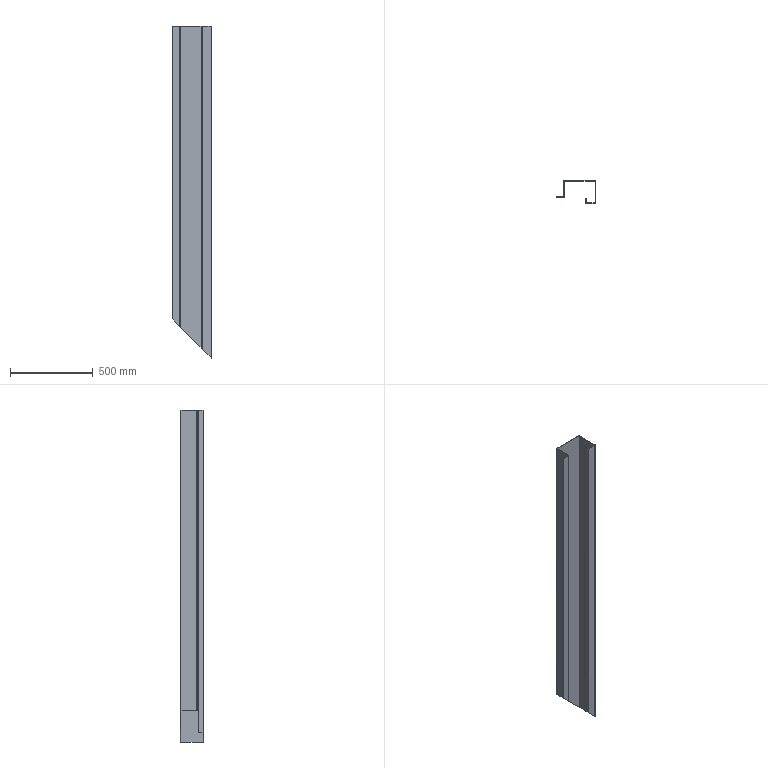Part | STEP file | TS-S79 | 1 solid | 50 faces | box 240 x 140 x 2010 mm | volume 3210076 mm3 | plane 31 | cylinder 14 | spline 5 | commonest cylinder face diameters 0.4 x5 6.4 x5 5 x4